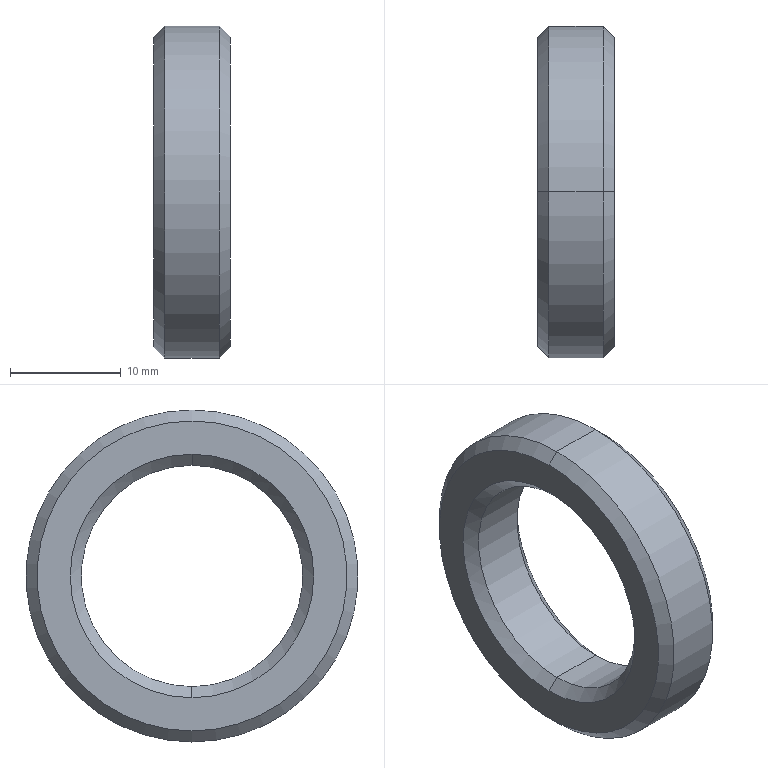Part | SolidWorks | features Chamfer 1, Extrusion 1 | 1 solid | 14 faces | box 6.9 x 30 x 30 mm | volume 2553 mm3 | cone 8 | cylinder 4 | plane 2 | commonest cylinder face diameters 20 x2 30 x2
STEP:
#1=CARTESIAN_POINT('',(5.9,0.,10.));
#2=VERTEX_POINT('',#1);
#3=CARTESIAN_POINT('',(5.9,0.,-10.));
#4=VERTEX_POINT('',#3);
#5=CARTESIAN_POINT('',(5.9,0.,0.));
#6=DIRECTION('',(1.,0.,0.));
#7=DIRECTION('',(0.,0.,-1.));
#8=AXIS2_PLACEMENT_3D('',#5,#6,#7);
#9=CIRCLE('',#8,10.);
#10=EDGE_CURVE('',#2,#4,#9,.T.);
#11=ORIENTED_EDGE('',*,*,#10,.F.);
#12=CARTESIAN_POINT('',(6.9,0.,11.));
#13=VERTEX_POINT('',#12);
#14=CARTESIAN_POINT('',(5.9,0.,10.));
#15=DIRECTION('',(0.7071,0.,0.7071));
#16=VECTOR('',#15,1000.);
#17=LINE('',#14,#16);
#18=EDGE_CURVE('',#2,#13,#17,.T.);
#19=ORIENTED_EDGE('',*,*,#18,.T.);
#20=CARTESIAN_POINT('',(6.9,0.,-11.));
#21=VERTEX_POINT('',#20);
#22=CARTESIAN_POINT('',(6.9,0.,0.));
#23=DIRECTION('',(-1.,0.,0.));
#24=DIRECTION('',(0.,0.,-1.));
#25=AXIS2_PLACEMENT_3D('',#22,#23,#24);
#26=CIRCLE('',#25,11.);
#27=EDGE_CURVE('',#21,#13,#26,.T.);
#28=ORIENTED_EDGE('',*,*,#27,.F.);
#29=CARTESIAN_POINT('',(5.9,0.,-10.));
#30=DIRECTION('',(0.7071,0.,-0.7071));
#31=VECTOR('',#30,1000.);
#32=LINE('',#29,#31);
#33=EDGE_CURVE('',#4,#21,#32,.T.);
#34=ORIENTED_EDGE('',*,*,#33,.F.);
#35=EDGE_LOOP('',(#11,#19,#28,#34));
#36=FACE_OUTER_BOUND('',#35,.T.);
#37=CARTESIAN_POINT('',(5.9,0.,0.));
#38=DIRECTION('',(1.,0.,0.));
#39=DIRECTION('',(0.,0.,-1.));
#40=AXIS2_PLACEMENT_3D('',#37,#38,#39);
#41=CONICAL_SURFACE('',#40,10.,0.7854);
#42=ADVANCED_FACE('',(#36),#41,.F.);
#43=CARTESIAN_POINT('',(1.,0.,-10.));
#44=VERTEX_POINT('',#43);
#45=CARTESIAN_POINT('',(1.,0.,10.));
#46=VERTEX_POINT('',#45);
#47=CARTESIAN_POINT('',(1.,0.,0.));
#48=DIRECTION('',(-1.,0.,0.));
#49=DIRECTION('',(0.,0.,-1.));
#50=AXIS2_PLACEMENT_3D('',#47,#48,#49);
#51=CIRCLE('',#50,10.);
#52=EDGE_CURVE('',#44,#46,#51,.T.);
#53=ORIENTED_EDGE('',*,*,#52,.F.);
#54=CARTESIAN_POINT('',(0.,0.,-11.));
#55=VERTEX_POINT('',#54);
#56=CARTESIAN_POINT('',(0.,0.,-11.));
#57=DIRECTION('',(-0.7071,0.,-0.7071));
#58=VECTOR('',#57,1000.);
#59=LINE('',#56,#58);
#60=EDGE_CURVE('',#44,#55,#59,.T.);
#61=ORIENTED_EDGE('',*,*,#60,.T.);
#62=CARTESIAN_POINT('',(0.,0.,11.));
#63=VERTEX_POINT('',#62);
#64=CARTESIAN_POINT('',(0.,0.,0.));
#65=DIRECTION('',(1.,0.,0.));
#66=DIRECTION('',(0.,0.,-1.));
#67=AXIS2_PLACEMENT_3D('',#64,#65,#66);
#68=CIRCLE('',#67,11.);
#69=EDGE_CURVE('',#63,#55,#68,.T.);
#70=ORIENTED_EDGE('',*,*,#69,.F.);
#71=CARTESIAN_POINT('',(0.,0.,11.));
#72=DIRECTION('',(-0.7071,0.,0.7071));
#73=VECTOR('',#72,1000.);
#74=LINE('',#71,#73);
#75=EDGE_CURVE('',#46,#63,#74,.T.);
#76=ORIENTED_EDGE('',*,*,#75,.F.);
#77=EDGE_LOOP('',(#53,#61,#70,#76));
#78=FACE_OUTER_BOUND('',#77,.T.);
#79=CARTESIAN_POINT('',(0.,0.,0.));
#80=DIRECTION('',(-1.,0.,0.));
#81=DIRECTION('',(0.,0.,1.));
#82=AXIS2_PLACEMENT_3D('',#79,#80,#81);
#83=CONICAL_SURFACE('',#82,11.,0.7854);
#84=ADVANCED_FACE('',(#78),#83,.F.);
#85=CARTESIAN_POINT('',(6.9,0.,-14.));
#86=VERTEX_POINT('',#85);
#87=CARTESIAN_POINT('',(6.9,0.,14.));
#88=VERTEX_POINT('',#87);
#89=CARTESIAN_POINT('',(6.9,0.,0.));
#90=DIRECTION('',(1.,0.,0.));
#91=DIRECTION('',(0.,0.,-1.));
#92=AXIS2_PLACEMENT_3D('',#89,#90,#91);
#93=CIRCLE('',#92,14.);
#94=EDGE_CURVE('',#86,#88,#93,.T.);
#95=ORIENTED_EDGE('',*,*,#94,.F.);
#96=CARTESIAN_POINT('',(5.9,0.,-15.));
#97=VERTEX_POINT('',#96);
#98=CARTESIAN_POINT('',(6.9,0.,-14.));
#99=DIRECTION('',(-0.7071,0.,-0.7071));
#100=VECTOR('',#99,1000.);
#101=LINE('',#98,#100);
#102=EDGE_CURVE('',#86,#97,#101,.T.);
#103=ORIENTED_EDGE('',*,*,#102,.T.);
#104=CARTESIAN_POINT('',(5.9,0.,15.));
#105=VERTEX_POINT('',#104);
#106=CARTESIAN_POINT('',(5.9,0.,0.));
#107=DIRECTION('',(-1.,0.,0.));
#108=DIRECTION('',(0.,0.,-1.));
#109=AXIS2_PLACEMENT_3D('',#106,#107,#108);
#110=CIRCLE('',#109,15.);
#111=EDGE_CURVE('',#105,#97,#110,.T.);
#112=ORIENTED_EDGE('',*,*,#111,.F.);
#113=CARTESIAN_POINT('',(6.9,0.,14.));
#114=DIRECTION('',(-0.7071,0.,0.7071));
#115=VECTOR('',#114,1000.);
#116=LINE('',#113,#115);
#117=EDGE_CURVE('',#88,#105,#116,.T.);
#118=ORIENTED_EDGE('',*,*,#117,.F.);
#119=EDGE_LOOP('',(#95,#103,#112,#118));
#120=FACE_OUTER_BOUND('',#119,.T.);
#121=CARTESIAN_POINT('',(6.9,0.,0.));
#122=DIRECTION('',(-1.,0.,0.));
#123=DIRECTION('',(0.,0.,1.));
#124=AXIS2_PLACEMENT_3D('',#121,#122,#123);
#125=CONICAL_SURFACE('',#124,14.,0.7854);
#126=ADVANCED_FACE('',(#120),#125,.T.);
#127=CARTESIAN_POINT('',(0.,0.,14.));
#128=VERTEX_POINT('',#127);
#129=CARTESIAN_POINT('',(0.,0.,-14.));
#130=VERTEX_POINT('',#129);
#131=CARTESIAN_POINT('',(0.,0.,0.));
#132=DIRECTION('',(-1.,0.,0.));
#133=DIRECTION('',(0.,0.,-1.));
#134=AXIS2_PLACEMENT_3D('',#131,#132,#133);
#135=CIRCLE('',#134,14.);
#136=EDGE_CURVE('',#128,#130,#135,.T.);
#137=ORIENTED_EDGE('',*,*,#136,.F.);
#138=CARTESIAN_POINT('',(1.,0.,15.));
#139=VERTEX_POINT('',#138);
#140=CARTESIAN_POINT('',(1.,0.,15.));
#141=DIRECTION('',(0.7071,0.,0.7071));
#142=VECTOR('',#141,1000.);
#143=LINE('',#140,#142);
#144=EDGE_CURVE('',#128,#139,#143,.T.);
#145=ORIENTED_EDGE('',*,*,#144,.T.);
#146=CARTESIAN_POINT('',(1.,0.,-15.));
#147=VERTEX_POINT('',#146);
#148=CARTESIAN_POINT('',(1.,0.,0.));
#149=DIRECTION('',(1.,0.,0.));
#150=DIRECTION('',(0.,0.,-1.));
#151=AXIS2_PLACEMENT_3D('',#148,#149,#150);
#152=CIRCLE('',#151,15.);
#153=EDGE_CURVE('',#147,#139,#152,.T.);
#154=ORIENTED_EDGE('',*,*,#153,.F.);
#155=CARTESIAN_POINT('',(1.,0.,-15.));
#156=DIRECTION('',(0.7071,0.,-0.7071));
#157=VECTOR('',#156,1000.);
#158=LINE('',#155,#157);
#159=EDGE_CURVE('',#130,#147,#158,.T.);
#160=ORIENTED_EDGE('',*,*,#159,.F.);
#161=EDGE_LOOP('',(#137,#145,#154,#160));
#162=FACE_OUTER_BOUND('',#161,.T.);
#163=CARTESIAN_POINT('',(1.,0.,0.));
#164=DIRECTION('',(1.,0.,0.));
#165=DIRECTION('',(0.,0.,-1.));
#166=AXIS2_PLACEMENT_3D('',#163,#164,#165);
#167=CONICAL_SURFACE('',#166,15.,0.7854);
#168=ADVANCED_FACE('',(#162),#167,.T.);
#169=ORIENTED_EDGE('',*,*,#10,.T.);
#170=CARTESIAN_POINT('',(6.9,0.,-10.));
#171=DIRECTION('',(-1.,0.,0.));
#172=VECTOR('',#171,1000.);
#173=LINE('',#170,#172);
#174=EDGE_CURVE('',#4,#44,#173,.T.);
#175=ORIENTED_EDGE('',*,*,#174,.T.);
#176=ORIENTED_EDGE('',*,*,#52,.T.);
#177=CARTESIAN_POINT('',(6.9,0.,10.));
#178=DIRECTION('',(-1.,0.,0.));
#179=VECTOR('',#178,1000.);
#180=LINE('',#177,#179);
#181=EDGE_CURVE('',#2,#46,#180,.T.);
#182=ORIENTED_EDGE('',*,*,#181,.F.);
#183=EDGE_LOOP('',(#169,#175,#176,#182));
#184=FACE_OUTER_BOUND('',#183,.T.);
#185=CARTESIAN_POINT('',(6.9,0.,0.));
#186=DIRECTION('',(-1.,0.,0.));
#187=DIRECTION('',(0.,0.,1.));
#188=AXIS2_PLACEMENT_3D('',#185,#186,#187);
#189=CYLINDRICAL_SURFACE('',#188,10.);
#190=ADVANCED_FACE('',(#184),#189,.F.);
#191=ORIENTED_EDGE('',*,*,#111,.T.);
#192=CARTESIAN_POINT('',(6.9,0.,-15.));
#193=DIRECTION('',(-1.,0.,0.));
#194=VECTOR('',#193,1000.);
#195=LINE('',#192,#194);
#196=EDGE_CURVE('',#97,#147,#195,.T.);
#197=ORIENTED_EDGE('',*,*,#196,.T.);
#198=ORIENTED_EDGE('',*,*,#153,.T.);
#199=CARTESIAN_POINT('',(6.9,0.,15.));
#200=DIRECTION('',(-1.,0.,0.));
#201=VECTOR('',#200,1000.);
#202=LINE('',#199,#201);
#203=EDGE_CURVE('',#105,#139,#202,.T.);
#204=ORIENTED_EDGE('',*,*,#203,.F.);
#205=EDGE_LOOP('',(#191,#197,#198,#204));
#206=FACE_OUTER_BOUND('',#205,.T.);
#207=CARTESIAN_POINT('',(6.9,0.,0.));
#208=DIRECTION('',(-1.,0.,0.));
#209=DIRECTION('',(0.,0.,1.));
#210=AXIS2_PLACEMENT_3D('',#207,#208,#209);
#211=CYLINDRICAL_SURFACE('',#210,15.);
#212=ADVANCED_FACE('',(#206),#211,.T.);
#213=CARTESIAN_POINT('',(6.9,0.,0.));
#214=DIRECTION('',(1.,0.,0.));
#215=DIRECTION('',(0.,0.,-1.));
#216=AXIS2_PLACEMENT_3D('',#213,#214,#215);
#217=CIRCLE('',#216,14.);
#218=EDGE_CURVE('',#88,#86,#217,.T.);
#219=ORIENTED_EDGE('',*,*,#218,.T.);
#220=ORIENTED_EDGE('',*,*,#94,.T.);
#221=EDGE_LOOP('',(#219,#220));
#222=FACE_OUTER_BOUND('',#221,.T.);
#223=ORIENTED_EDGE('',*,*,#27,.T.);
#224=CARTESIAN_POINT('',(6.9,0.,0.));
#225=DIRECTION('',(-1.,0.,0.));
#226=DIRECTION('',(0.,0.,-1.));
#227=AXIS2_PLACEMENT_3D('',#224,#225,#226);
#228=CIRCLE('',#227,11.);
#229=EDGE_CURVE('',#13,#21,#228,.T.);
#230=ORIENTED_EDGE('',*,*,#229,.T.);
#231=EDGE_LOOP('',(#223,#230));
#232=FACE_BOUND('',#231,.T.);
#233=CARTESIAN_POINT('',(6.9,0.,0.));
#234=DIRECTION('',(1.,0.,0.));
#235=DIRECTION('',(0.,0.,-1.));
#236=AXIS2_PLACEMENT_3D('',#233,#234,#235);
#237=PLANE('',#236);
#238=ADVANCED_FACE('',(#222,#232),#237,.T.);
#239=CARTESIAN_POINT('',(0.,0.,0.));
#240=DIRECTION('',(-1.,0.,0.));
#241=DIRECTION('',(0.,0.,-1.));
#242=AXIS2_PLACEMENT_3D('',#239,#240,#241);
#243=CIRCLE('',#242,14.);
#244=EDGE_CURVE('',#130,#128,#243,.T.);
#245=ORIENTED_EDGE('',*,*,#244,.T.);
#246=ORIENTED_EDGE('',*,*,#136,.T.);
#247=EDGE_LOOP('',(#245,#246));
#248=FACE_OUTER_BOUND('',#247,.T.);
#249=ORIENTED_EDGE('',*,*,#69,.T.);
#250=CARTESIAN_POINT('',(0.,0.,0.));
#251=DIRECTION('',(1.,0.,0.));
#252=DIRECTION('',(0.,0.,-1.));
#253=AXIS2_PLACEMENT_3D('',#250,#251,#252);
#254=CIRCLE('',#253,11.);
#255=EDGE_CURVE('',#55,#63,#254,.T.);
#256=ORIENTED_EDGE('',*,*,#255,.T.);
#257=EDGE_LOOP('',(#249,#256));
#258=FACE_BOUND('',#257,.T.);
#259=CARTESIAN_POINT('',(0.,0.,0.));
#260=DIRECTION('',(1.,0.,0.));
#261=DIRECTION('',(0.,0.,-1.));
#262=AXIS2_PLACEMENT_3D('',#259,#260,#261);
#263=PLANE('',#262);
#264=ADVANCED_FACE('',(#248,#258),#263,.F.);
#265=ORIENTED_EDGE('',*,*,#196,.F.);
#266=CARTESIAN_POINT('',(5.9,0.,0.));
#267=DIRECTION('',(-1.,0.,0.));
#268=DIRECTION('',(0.,0.,-1.));
#269=AXIS2_PLACEMENT_3D('',#266,#267,#268);
#270=CIRCLE('',#269,15.);
#271=EDGE_CURVE('',#97,#105,#270,.T.);
#272=ORIENTED_EDGE('',*,*,#271,.T.);
#273=ORIENTED_EDGE('',*,*,#203,.T.);
#274=CARTESIAN_POINT('',(1.,0.,0.));
#275=DIRECTION('',(1.,0.,0.));
#276=DIRECTION('',(0.,0.,-1.));
#277=AXIS2_PLACEMENT_3D('',#274,#275,#276);
#278=CIRCLE('',#277,15.);
#279=EDGE_CURVE('',#139,#147,#278,.T.);
#280=ORIENTED_EDGE('',*,*,#279,.T.);
#281=EDGE_LOOP('',(#265,#272,#273,#280));
#282=FACE_OUTER_BOUND('',#281,.T.);
#283=CARTESIAN_POINT('',(6.9,0.,0.));
#284=DIRECTION('',(-1.,0.,0.));
#285=DIRECTION('',(0.,0.,1.));
#286=AXIS2_PLACEMENT_3D('',#283,#284,#285);
#287=CYLINDRICAL_SURFACE('',#286,15.);
#288=ADVANCED_FACE('',(#282),#287,.T.);
#289=ORIENTED_EDGE('',*,*,#174,.F.);
#290=CARTESIAN_POINT('',(5.9,0.,0.));
#291=DIRECTION('',(1.,0.,0.));
#292=DIRECTION('',(0.,0.,-1.));
#293=AXIS2_PLACEMENT_3D('',#290,#291,#292);
#294=CIRCLE('',#293,10.);
#295=EDGE_CURVE('',#4,#2,#294,.T.);
#296=ORIENTED_EDGE('',*,*,#295,.T.);
#297=ORIENTED_EDGE('',*,*,#181,.T.);
#298=CARTESIAN_POINT('',(1.,0.,0.));
#299=DIRECTION('',(-1.,0.,0.));
#300=DIRECTION('',(0.,0.,-1.));
#301=AXIS2_PLACEMENT_3D('',#298,#299,#300);
#302=CIRCLE('',#301,10.);
#303=EDGE_CURVE('',#46,#44,#302,.T.);
#304=ORIENTED_EDGE('',*,*,#303,.T.);
#305=EDGE_LOOP('',(#289,#296,#297,#304));
#306=FACE_OUTER_BOUND('',#305,.T.);
#307=CARTESIAN_POINT('',(6.9,0.,0.));
#308=DIRECTION('',(-1.,0.,0.));
#309=DIRECTION('',(0.,0.,1.));
#310=AXIS2_PLACEMENT_3D('',#307,#308,#309);
#311=CYLINDRICAL_SURFACE('',#310,10.);
#312=ADVANCED_FACE('',(#306),#311,.F.);
#313=ORIENTED_EDGE('',*,*,#144,.F.);
#314=ORIENTED_EDGE('',*,*,#244,.F.);
#315=ORIENTED_EDGE('',*,*,#159,.T.);
#316=ORIENTED_EDGE('',*,*,#279,.F.);
#317=EDGE_LOOP('',(#313,#314,#315,#316));
#318=FACE_OUTER_BOUND('',#317,.T.);
#319=CARTESIAN_POINT('',(1.,0.,0.));
#320=DIRECTION('',(1.,0.,0.));
#321=DIRECTION('',(0.,0.,-1.));
#322=AXIS2_PLACEMENT_3D('',#319,#320,#321);
#323=CONICAL_SURFACE('',#322,15.,0.7854);
#324=ADVANCED_FACE('',(#318),#323,.T.);
#325=ORIENTED_EDGE('',*,*,#102,.F.);
#326=ORIENTED_EDGE('',*,*,#218,.F.);
#327=ORIENTED_EDGE('',*,*,#117,.T.);
#328=ORIENTED_EDGE('',*,*,#271,.F.);
#329=EDGE_LOOP('',(#325,#326,#327,#328));
#330=FACE_OUTER_BOUND('',#329,.T.);
#331=CARTESIAN_POINT('',(6.9,0.,0.));
#332=DIRECTION('',(-1.,0.,0.));
#333=DIRECTION('',(0.,0.,1.));
#334=AXIS2_PLACEMENT_3D('',#331,#332,#333);
#335=CONICAL_SURFACE('',#334,14.,0.7854);
#336=ADVANCED_FACE('',(#330),#335,.T.);
#337=ORIENTED_EDGE('',*,*,#60,.F.);
#338=ORIENTED_EDGE('',*,*,#303,.F.);
#339=ORIENTED_EDGE('',*,*,#75,.T.);
#340=ORIENTED_EDGE('',*,*,#255,.F.);
#341=EDGE_LOOP('',(#337,#338,#339,#340));
#342=FACE_OUTER_BOUND('',#341,.T.);
#343=CARTESIAN_POINT('',(0.,0.,0.));
#344=DIRECTION('',(-1.,0.,0.));
#345=DIRECTION('',(0.,0.,1.));
#346=AXIS2_PLACEMENT_3D('',#343,#344,#345);
#347=CONICAL_SURFACE('',#346,11.,0.7854);
#348=ADVANCED_FACE('',(#342),#347,.F.);
#349=ORIENTED_EDGE('',*,*,#18,.F.);
#350=ORIENTED_EDGE('',*,*,#295,.F.);
#351=ORIENTED_EDGE('',*,*,#33,.T.);
#352=ORIENTED_EDGE('',*,*,#229,.F.);
#353=EDGE_LOOP('',(#349,#350,#351,#352));
#354=FACE_OUTER_BOUND('',#353,.T.);
#355=CARTESIAN_POINT('',(5.9,0.,0.));
#356=DIRECTION('',(1.,0.,0.));
#357=DIRECTION('',(0.,0.,-1.));
#358=AXIS2_PLACEMENT_3D('',#355,#356,#357);
#359=CONICAL_SURFACE('',#358,10.,0.7854);
#360=ADVANCED_FACE('',(#354),#359,.F.);
#361=CLOSED_SHELL('',(#42,#84,#126,#168,#190,#212,#238,#264,#288,#312,#324,#336,#348,#360));
#362=MANIFOLD_SOLID_BREP('',#361);
#363=CARTESIAN_POINT('',(0.,0.,0.));
#364=DIRECTION('',(0.,0.,1.));
#365=DIRECTION('',(1.,0.,0.));
#366=AXIS2_PLACEMENT_3D('',#363,#364,#365);
#367=(LENGTH_UNIT()NAMED_UNIT(*)SI_UNIT(.MILLI.,.METRE.));
#368=UNCERTAINTY_MEASURE_WITH_UNIT(LENGTH_MEASURE(0.00001),#367,'','');
#369=(NAMED_UNIT(*)PLANE_ANGLE_UNIT()SI_UNIT($,.RADIAN.));
#370=(NAMED_UNIT(*)SI_UNIT($,.STERADIAN.)SOLID_ANGLE_UNIT());
#371=(GEOMETRIC_REPRESENTATION_CONTEXT(3)GLOBAL_UNCERTAINTY_ASSIGNED_CONTEXT((#368))GLOBAL_UNIT_ASSIGNED_CONTEXT((#367,#369,#370))REPRESENTATION_CONTEXT('',''));
#372=ADVANCED_BREP_SHAPE_REPRESENTATION('',(#362,#366),#371);